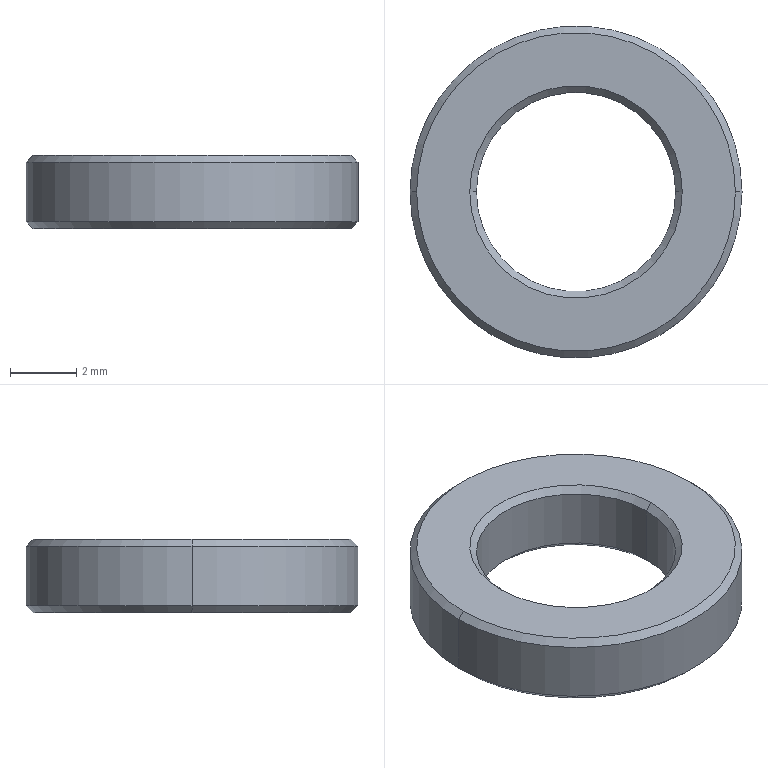Part | NX | features BREP 1 | 1 solid | 14 faces | box 10 x 10 x 2.2 mm | volume 108.573 mm3 | cone 8 | cylinder 4 | plane 2 | commonest cylinder face diameters 6 x2 10 x2
STEP:
#1=CARTESIAN_POINT('',(4.8,0.,1.1));
#2=VERTEX_POINT('',#1);
#3=CARTESIAN_POINT('',(5.,0.,0.9));
#4=VERTEX_POINT('',#3);
#5=CARTESIAN_POINT('',(4.8,0.,1.1));
#6=DIRECTION('',(0.7071,0.,-0.7071));
#7=VECTOR('',#6,1000.);
#8=LINE('',#5,#7);
#9=EDGE_CURVE('',#2,#4,#8,.T.);
#10=ORIENTED_EDGE('',*,*,#9,.F.);
#11=CARTESIAN_POINT('',(-4.8,0.,1.1));
#12=VERTEX_POINT('',#11);
#13=CARTESIAN_POINT('',(0.,0.,1.1));
#14=DIRECTION('',(0.,0.,1.));
#15=DIRECTION('',(1.,0.,0.));
#16=AXIS2_PLACEMENT_3D('',#13,#14,#15);
#17=CIRCLE('',#16,4.8);
#18=EDGE_CURVE('',#12,#2,#17,.T.);
#19=ORIENTED_EDGE('',*,*,#18,.F.);
#20=CARTESIAN_POINT('',(-5.,0.,0.9));
#21=VERTEX_POINT('',#20);
#22=CARTESIAN_POINT('',(-4.8,0.,1.1));
#23=DIRECTION('',(-0.7071,0.,-0.7071));
#24=VECTOR('',#23,1000.);
#25=LINE('',#22,#24);
#26=EDGE_CURVE('',#12,#21,#25,.T.);
#27=ORIENTED_EDGE('',*,*,#26,.T.);
#28=CARTESIAN_POINT('',(0.,0.,0.9));
#29=DIRECTION('',(0.,0.,-1.));
#30=DIRECTION('',(1.,0.,0.));
#31=AXIS2_PLACEMENT_3D('',#28,#29,#30);
#32=CIRCLE('',#31,5.);
#33=EDGE_CURVE('',#4,#21,#32,.T.);
#34=ORIENTED_EDGE('',*,*,#33,.F.);
#35=EDGE_LOOP('',(#10,#19,#27,#34));
#36=FACE_BOUND('',#35,.T.);
#37=CARTESIAN_POINT('',(0.,0.,1.1));
#38=DIRECTION('',(0.,0.,-1.));
#39=DIRECTION('',(-1.,0.,0.));
#40=AXIS2_PLACEMENT_3D('',#37,#38,#39);
#41=CONICAL_SURFACE('',#40,4.8,0.7854);
#42=ADVANCED_FACE('',(#36),#41,.T.);
#43=CARTESIAN_POINT('',(-5.,0.,-0.9));
#44=VERTEX_POINT('',#43);
#45=CARTESIAN_POINT('',(-4.8,0.,-1.1));
#46=VERTEX_POINT('',#45);
#47=CARTESIAN_POINT('',(-5.,0.,-0.9));
#48=DIRECTION('',(-0.7071,0.,0.7071));
#49=VECTOR('',#48,1000.);
#50=LINE('',#47,#49);
#51=EDGE_CURVE('',#44,#46,#50,.F.);
#52=ORIENTED_EDGE('',*,*,#51,.T.);
#53=CARTESIAN_POINT('',(4.8,0.,-1.1));
#54=VERTEX_POINT('',#53);
#55=CARTESIAN_POINT('',(0.,0.,-1.1));
#56=DIRECTION('',(0.,0.,-1.));
#57=DIRECTION('',(1.,0.,0.));
#58=AXIS2_PLACEMENT_3D('',#55,#56,#57);
#59=CIRCLE('',#58,4.8);
#60=EDGE_CURVE('',#54,#46,#59,.T.);
#61=ORIENTED_EDGE('',*,*,#60,.F.);
#62=CARTESIAN_POINT('',(5.,0.,-0.9));
#63=VERTEX_POINT('',#62);
#64=CARTESIAN_POINT('',(5.,0.,-0.9));
#65=DIRECTION('',(0.7071,0.,0.7071));
#66=VECTOR('',#65,1000.);
#67=LINE('',#64,#66);
#68=EDGE_CURVE('',#63,#54,#67,.F.);
#69=ORIENTED_EDGE('',*,*,#68,.F.);
#70=CARTESIAN_POINT('',(0.,0.,-0.9));
#71=DIRECTION('',(0.,0.,1.));
#72=DIRECTION('',(1.,0.,0.));
#73=AXIS2_PLACEMENT_3D('',#70,#71,#72);
#74=CIRCLE('',#73,5.);
#75=EDGE_CURVE('',#44,#63,#74,.T.);
#76=ORIENTED_EDGE('',*,*,#75,.F.);
#77=EDGE_LOOP('',(#52,#61,#69,#76));
#78=FACE_BOUND('',#77,.T.);
#79=CARTESIAN_POINT('',(0.,0.,-0.9));
#80=DIRECTION('',(0.,0.,1.));
#81=DIRECTION('',(1.,0.,0.));
#82=AXIS2_PLACEMENT_3D('',#79,#80,#81);
#83=CONICAL_SURFACE('',#82,5.,0.7854);
#84=ADVANCED_FACE('',(#78),#83,.T.);
#85=CARTESIAN_POINT('',(-3.2,0.,1.1));
#86=VERTEX_POINT('',#85);
#87=CARTESIAN_POINT('',(-3.,0.,0.9));
#88=VERTEX_POINT('',#87);
#89=CARTESIAN_POINT('',(-3.,0.,0.9));
#90=DIRECTION('',(-0.7071,0.,0.7071));
#91=VECTOR('',#90,1000.);
#92=LINE('',#89,#91);
#93=EDGE_CURVE('',#86,#88,#92,.F.);
#94=ORIENTED_EDGE('',*,*,#93,.T.);
#95=CARTESIAN_POINT('',(3.,0.,0.9));
#96=VERTEX_POINT('',#95);
#97=CARTESIAN_POINT('',(0.,0.,0.9));
#98=DIRECTION('',(0.,0.,1.));
#99=DIRECTION('',(1.,0.,0.));
#100=AXIS2_PLACEMENT_3D('',#97,#98,#99);
#101=CIRCLE('',#100,3.);
#102=EDGE_CURVE('',#96,#88,#101,.T.);
#103=ORIENTED_EDGE('',*,*,#102,.F.);
#104=CARTESIAN_POINT('',(3.2,0.,1.1));
#105=VERTEX_POINT('',#104);
#106=CARTESIAN_POINT('',(3.,0.,0.9));
#107=DIRECTION('',(0.7071,0.,0.7071));
#108=VECTOR('',#107,1000.);
#109=LINE('',#106,#108);
#110=EDGE_CURVE('',#105,#96,#109,.F.);
#111=ORIENTED_EDGE('',*,*,#110,.F.);
#112=CARTESIAN_POINT('',(0.,0.,1.1));
#113=DIRECTION('',(0.,0.,-1.));
#114=DIRECTION('',(1.,0.,0.));
#115=AXIS2_PLACEMENT_3D('',#112,#113,#114);
#116=CIRCLE('',#115,3.2);
#117=EDGE_CURVE('',#86,#105,#116,.T.);
#118=ORIENTED_EDGE('',*,*,#117,.F.);
#119=EDGE_LOOP('',(#94,#103,#111,#118));
#120=FACE_BOUND('',#119,.T.);
#121=CARTESIAN_POINT('',(0.,0.,0.9));
#122=DIRECTION('',(0.,0.,1.));
#123=DIRECTION('',(1.,0.,0.));
#124=AXIS2_PLACEMENT_3D('',#121,#122,#123);
#125=CONICAL_SURFACE('',#124,3.,0.7854);
#126=ADVANCED_FACE('',(#120),#125,.F.);
#127=CARTESIAN_POINT('',(3.,0.,-0.9));
#128=VERTEX_POINT('',#127);
#129=CARTESIAN_POINT('',(3.2,0.,-1.1));
#130=VERTEX_POINT('',#129);
#131=CARTESIAN_POINT('',(3.2,0.,-1.1));
#132=DIRECTION('',(0.7071,0.,-0.7071));
#133=VECTOR('',#132,1000.);
#134=LINE('',#131,#133);
#135=EDGE_CURVE('',#128,#130,#134,.T.);
#136=ORIENTED_EDGE('',*,*,#135,.F.);
#137=CARTESIAN_POINT('',(-3.,0.,-0.9));
#138=VERTEX_POINT('',#137);
#139=CARTESIAN_POINT('',(0.,0.,-0.9));
#140=DIRECTION('',(0.,0.,-1.));
#141=DIRECTION('',(1.,0.,0.));
#142=AXIS2_PLACEMENT_3D('',#139,#140,#141);
#143=CIRCLE('',#142,3.);
#144=EDGE_CURVE('',#138,#128,#143,.T.);
#145=ORIENTED_EDGE('',*,*,#144,.F.);
#146=CARTESIAN_POINT('',(-3.2,0.,-1.1));
#147=VERTEX_POINT('',#146);
#148=CARTESIAN_POINT('',(-3.2,0.,-1.1));
#149=DIRECTION('',(-0.7071,0.,-0.7071));
#150=VECTOR('',#149,1000.);
#151=LINE('',#148,#150);
#152=EDGE_CURVE('',#138,#147,#151,.T.);
#153=ORIENTED_EDGE('',*,*,#152,.T.);
#154=CARTESIAN_POINT('',(0.,0.,-1.1));
#155=DIRECTION('',(0.,0.,1.));
#156=DIRECTION('',(1.,0.,0.));
#157=AXIS2_PLACEMENT_3D('',#154,#155,#156);
#158=CIRCLE('',#157,3.2);
#159=EDGE_CURVE('',#130,#147,#158,.T.);
#160=ORIENTED_EDGE('',*,*,#159,.F.);
#161=EDGE_LOOP('',(#136,#145,#153,#160));
#162=FACE_BOUND('',#161,.T.);
#163=CARTESIAN_POINT('',(0.,0.,-1.1));
#164=DIRECTION('',(0.,0.,-1.));
#165=DIRECTION('',(-1.,0.,0.));
#166=AXIS2_PLACEMENT_3D('',#163,#164,#165);
#167=CONICAL_SURFACE('',#166,3.2,0.7854);
#168=ADVANCED_FACE('',(#162),#167,.F.);
#169=CARTESIAN_POINT('',(3.,0.,1.1));
#170=DIRECTION('',(0.,0.,-1.));
#171=VECTOR('',#170,1000.);
#172=LINE('',#169,#171);
#173=EDGE_CURVE('',#96,#128,#172,.T.);
#174=ORIENTED_EDGE('',*,*,#173,.F.);
#175=ORIENTED_EDGE('',*,*,#102,.T.);
#176=CARTESIAN_POINT('',(-3.,0.,1.1));
#177=DIRECTION('',(0.,0.,-1.));
#178=VECTOR('',#177,1000.);
#179=LINE('',#176,#178);
#180=EDGE_CURVE('',#88,#138,#179,.T.);
#181=ORIENTED_EDGE('',*,*,#180,.T.);
#182=ORIENTED_EDGE('',*,*,#144,.T.);
#183=EDGE_LOOP('',(#174,#175,#181,#182));
#184=FACE_BOUND('',#183,.T.);
#185=CARTESIAN_POINT('',(0.,0.,1.1));
#186=DIRECTION('',(0.,0.,-1.));
#187=DIRECTION('',(-1.,0.,0.));
#188=AXIS2_PLACEMENT_3D('',#185,#186,#187);
#189=CYLINDRICAL_SURFACE('',#188,3.);
#190=ADVANCED_FACE('',(#184),#189,.F.);
#191=CARTESIAN_POINT('',(5.,0.,1.1));
#192=DIRECTION('',(0.,0.,-1.));
#193=VECTOR('',#192,1000.);
#194=LINE('',#191,#193);
#195=EDGE_CURVE('',#4,#63,#194,.T.);
#196=ORIENTED_EDGE('',*,*,#195,.F.);
#197=ORIENTED_EDGE('',*,*,#33,.T.);
#198=CARTESIAN_POINT('',(-5.,0.,1.1));
#199=DIRECTION('',(0.,0.,-1.));
#200=VECTOR('',#199,1000.);
#201=LINE('',#198,#200);
#202=EDGE_CURVE('',#21,#44,#201,.T.);
#203=ORIENTED_EDGE('',*,*,#202,.T.);
#204=ORIENTED_EDGE('',*,*,#75,.T.);
#205=EDGE_LOOP('',(#196,#197,#203,#204));
#206=FACE_BOUND('',#205,.T.);
#207=CARTESIAN_POINT('',(0.,0.,1.1));
#208=DIRECTION('',(0.,0.,-1.));
#209=DIRECTION('',(-1.,0.,0.));
#210=AXIS2_PLACEMENT_3D('',#207,#208,#209);
#211=CYLINDRICAL_SURFACE('',#210,5.);
#212=ADVANCED_FACE('',(#206),#211,.T.);
#213=ORIENTED_EDGE('',*,*,#60,.T.);
#214=CARTESIAN_POINT('',(0.,0.,-1.1));
#215=DIRECTION('',(0.,0.,-1.));
#216=DIRECTION('',(1.,0.,0.));
#217=AXIS2_PLACEMENT_3D('',#214,#215,#216);
#218=CIRCLE('',#217,4.8);
#219=EDGE_CURVE('',#46,#54,#218,.T.);
#220=ORIENTED_EDGE('',*,*,#219,.T.);
#221=EDGE_LOOP('',(#213,#220));
#222=FACE_BOUND('',#221,.T.);
#223=CARTESIAN_POINT('',(0.,0.,-1.1));
#224=DIRECTION('',(0.,0.,1.));
#225=DIRECTION('',(1.,0.,0.));
#226=AXIS2_PLACEMENT_3D('',#223,#224,#225);
#227=CIRCLE('',#226,3.2);
#228=EDGE_CURVE('',#147,#130,#227,.T.);
#229=ORIENTED_EDGE('',*,*,#228,.T.);
#230=ORIENTED_EDGE('',*,*,#159,.T.);
#231=EDGE_LOOP('',(#229,#230));
#232=FACE_BOUND('',#231,.T.);
#233=CARTESIAN_POINT('',(0.,0.,-1.1));
#234=DIRECTION('',(0.,0.,1.));
#235=DIRECTION('',(1.,0.,0.));
#236=AXIS2_PLACEMENT_3D('',#233,#234,#235);
#237=PLANE('',#236);
#238=ADVANCED_FACE('',(#222,#232),#237,.F.);
#239=ORIENTED_EDGE('',*,*,#18,.T.);
#240=CARTESIAN_POINT('',(0.,0.,1.1));
#241=DIRECTION('',(0.,0.,1.));
#242=DIRECTION('',(1.,0.,0.));
#243=AXIS2_PLACEMENT_3D('',#240,#241,#242);
#244=CIRCLE('',#243,4.8);
#245=EDGE_CURVE('',#2,#12,#244,.T.);
#246=ORIENTED_EDGE('',*,*,#245,.T.);
#247=EDGE_LOOP('',(#239,#246));
#248=FACE_BOUND('',#247,.T.);
#249=CARTESIAN_POINT('',(0.,0.,1.1));
#250=DIRECTION('',(0.,0.,-1.));
#251=DIRECTION('',(1.,0.,0.));
#252=AXIS2_PLACEMENT_3D('',#249,#250,#251);
#253=CIRCLE('',#252,3.2);
#254=EDGE_CURVE('',#105,#86,#253,.T.);
#255=ORIENTED_EDGE('',*,*,#254,.T.);
#256=ORIENTED_EDGE('',*,*,#117,.T.);
#257=EDGE_LOOP('',(#255,#256));
#258=FACE_BOUND('',#257,.T.);
#259=CARTESIAN_POINT('',(0.,0.,1.1));
#260=DIRECTION('',(0.,0.,1.));
#261=DIRECTION('',(1.,0.,0.));
#262=AXIS2_PLACEMENT_3D('',#259,#260,#261);
#263=PLANE('',#262);
#264=ADVANCED_FACE('',(#248,#258),#263,.T.);
#265=CARTESIAN_POINT('',(0.,0.,0.9));
#266=DIRECTION('',(0.,0.,-1.));
#267=DIRECTION('',(1.,0.,0.));
#268=AXIS2_PLACEMENT_3D('',#265,#266,#267);
#269=CIRCLE('',#268,5.);
#270=EDGE_CURVE('',#21,#4,#269,.T.);
#271=ORIENTED_EDGE('',*,*,#270,.T.);
#272=ORIENTED_EDGE('',*,*,#195,.T.);
#273=CARTESIAN_POINT('',(0.,0.,-0.9));
#274=DIRECTION('',(0.,0.,1.));
#275=DIRECTION('',(1.,0.,0.));
#276=AXIS2_PLACEMENT_3D('',#273,#274,#275);
#277=CIRCLE('',#276,5.);
#278=EDGE_CURVE('',#63,#44,#277,.T.);
#279=ORIENTED_EDGE('',*,*,#278,.T.);
#280=ORIENTED_EDGE('',*,*,#202,.F.);
#281=EDGE_LOOP('',(#271,#272,#279,#280));
#282=FACE_BOUND('',#281,.T.);
#283=CARTESIAN_POINT('',(0.,0.,1.1));
#284=DIRECTION('',(0.,0.,-1.));
#285=DIRECTION('',(-1.,0.,0.));
#286=AXIS2_PLACEMENT_3D('',#283,#284,#285);
#287=CYLINDRICAL_SURFACE('',#286,5.);
#288=ADVANCED_FACE('',(#282),#287,.T.);
#289=CARTESIAN_POINT('',(0.,0.,0.9));
#290=DIRECTION('',(0.,0.,1.));
#291=DIRECTION('',(1.,0.,0.));
#292=AXIS2_PLACEMENT_3D('',#289,#290,#291);
#293=CIRCLE('',#292,3.);
#294=EDGE_CURVE('',#88,#96,#293,.T.);
#295=ORIENTED_EDGE('',*,*,#294,.T.);
#296=ORIENTED_EDGE('',*,*,#173,.T.);
#297=CARTESIAN_POINT('',(0.,0.,-0.9));
#298=DIRECTION('',(0.,0.,-1.));
#299=DIRECTION('',(1.,0.,0.));
#300=AXIS2_PLACEMENT_3D('',#297,#298,#299);
#301=CIRCLE('',#300,3.);
#302=EDGE_CURVE('',#128,#138,#301,.T.);
#303=ORIENTED_EDGE('',*,*,#302,.T.);
#304=ORIENTED_EDGE('',*,*,#180,.F.);
#305=EDGE_LOOP('',(#295,#296,#303,#304));
#306=FACE_BOUND('',#305,.T.);
#307=CARTESIAN_POINT('',(0.,0.,1.1));
#308=DIRECTION('',(0.,0.,-1.));
#309=DIRECTION('',(-1.,0.,0.));
#310=AXIS2_PLACEMENT_3D('',#307,#308,#309);
#311=CYLINDRICAL_SURFACE('',#310,3.);
#312=ADVANCED_FACE('',(#306),#311,.F.);
#313=ORIENTED_EDGE('',*,*,#302,.F.);
#314=ORIENTED_EDGE('',*,*,#135,.T.);
#315=ORIENTED_EDGE('',*,*,#228,.F.);
#316=ORIENTED_EDGE('',*,*,#152,.F.);
#317=EDGE_LOOP('',(#313,#314,#315,#316));
#318=FACE_BOUND('',#317,.T.);
#319=CARTESIAN_POINT('',(0.,0.,-1.1));
#320=DIRECTION('',(0.,0.,-1.));
#321=DIRECTION('',(-1.,0.,0.));
#322=AXIS2_PLACEMENT_3D('',#319,#320,#321);
#323=CONICAL_SURFACE('',#322,3.2,0.7854);
#324=ADVANCED_FACE('',(#318),#323,.F.);
#325=ORIENTED_EDGE('',*,*,#294,.F.);
#326=ORIENTED_EDGE('',*,*,#93,.F.);
#327=ORIENTED_EDGE('',*,*,#254,.F.);
#328=ORIENTED_EDGE('',*,*,#110,.T.);
#329=EDGE_LOOP('',(#325,#326,#327,#328));
#330=FACE_BOUND('',#329,.T.);
#331=CARTESIAN_POINT('',(0.,0.,0.9));
#332=DIRECTION('',(0.,0.,1.));
#333=DIRECTION('',(1.,0.,0.));
#334=AXIS2_PLACEMENT_3D('',#331,#332,#333);
#335=CONICAL_SURFACE('',#334,3.,0.7854);
#336=ADVANCED_FACE('',(#330),#335,.F.);
#337=ORIENTED_EDGE('',*,*,#219,.F.);
#338=ORIENTED_EDGE('',*,*,#51,.F.);
#339=ORIENTED_EDGE('',*,*,#278,.F.);
#340=ORIENTED_EDGE('',*,*,#68,.T.);
#341=EDGE_LOOP('',(#337,#338,#339,#340));
#342=FACE_BOUND('',#341,.T.);
#343=CARTESIAN_POINT('',(0.,0.,-0.9));
#344=DIRECTION('',(0.,0.,1.));
#345=DIRECTION('',(1.,0.,0.));
#346=AXIS2_PLACEMENT_3D('',#343,#344,#345);
#347=CONICAL_SURFACE('',#346,5.,0.7854);
#348=ADVANCED_FACE('',(#342),#347,.T.);
#349=ORIENTED_EDGE('',*,*,#245,.F.);
#350=ORIENTED_EDGE('',*,*,#9,.T.);
#351=ORIENTED_EDGE('',*,*,#270,.F.);
#352=ORIENTED_EDGE('',*,*,#26,.F.);
#353=EDGE_LOOP('',(#349,#350,#351,#352));
#354=FACE_BOUND('',#353,.T.);
#355=CARTESIAN_POINT('',(0.,0.,1.1));
#356=DIRECTION('',(0.,0.,-1.));
#357=DIRECTION('',(-1.,0.,0.));
#358=AXIS2_PLACEMENT_3D('',#355,#356,#357);
#359=CONICAL_SURFACE('',#358,4.8,0.7854);
#360=ADVANCED_FACE('',(#354),#359,.T.);
#361=CLOSED_SHELL('',(#42,#84,#126,#168,#190,#212,#238,#264,#288,#312,#324,#336,#348,#360));
#362=MANIFOLD_SOLID_BREP('',#361);
#363=(LENGTH_UNIT()NAMED_UNIT(*)SI_UNIT(.MILLI.,.METRE.));
#364=UNCERTAINTY_MEASURE_WITH_UNIT(LENGTH_MEASURE(0.00001),#363,'','');
#365=(NAMED_UNIT(*)PLANE_ANGLE_UNIT()SI_UNIT($,.RADIAN.));
#366=(NAMED_UNIT(*)SI_UNIT($,.STERADIAN.)SOLID_ANGLE_UNIT());
#367=(GEOMETRIC_REPRESENTATION_CONTEXT(3)GLOBAL_UNCERTAINTY_ASSIGNED_CONTEXT((#364))GLOBAL_UNIT_ASSIGNED_CONTEXT((#363,#365,#366))REPRESENTATION_CONTEXT('',''));
#368=ADVANCED_BREP_SHAPE_REPRESENTATION('',(#362),#367);